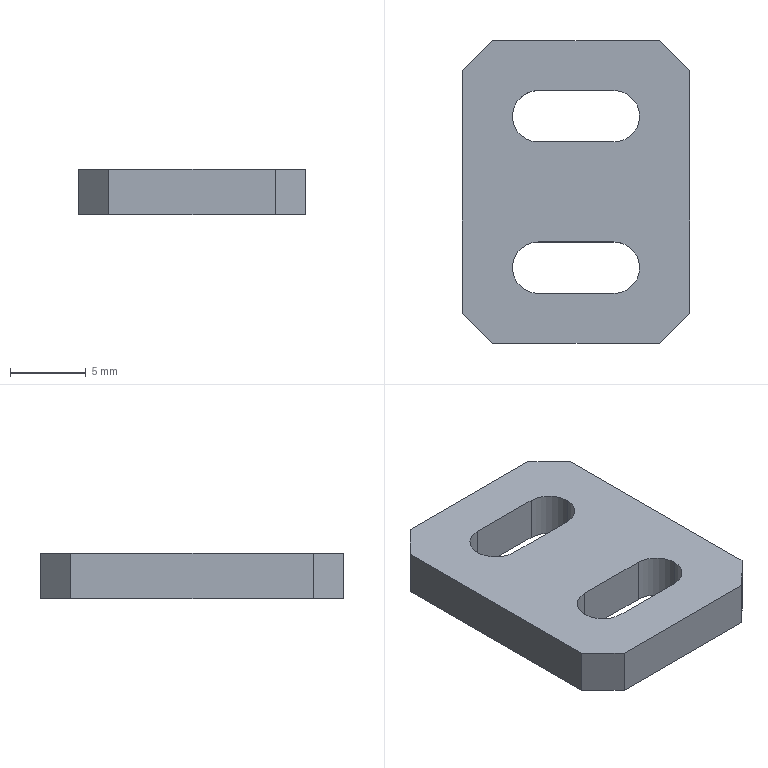Part | SolidWorks | features Chamfer 1, Extrusion 1, HoleWzd 1 | 1 solid | 20 faces | box 15 x 20 x 3 mm | volume 719.525 mm3 | plane 14 | cylinder 6 | commonest cylinder face diameters 3.4 x6
STEP:
#1=CARTESIAN_POINT('',(4.2,5.,0.));
#2=VERTEX_POINT('',#1);
#3=CARTESIAN_POINT('',(2.5,6.7,0.));
#4=VERTEX_POINT('',#3);
#5=CARTESIAN_POINT('',(2.5,5.,0.));
#6=DIRECTION('',(0.,0.,1.));
#7=DIRECTION('',(1.,0.,0.));
#8=AXIS2_PLACEMENT_3D('',#5,#6,#7);
#9=CIRCLE('',#8,1.7);
#10=EDGE_CURVE('',#2,#4,#9,.T.);
#11=ORIENTED_EDGE('',*,*,#10,.F.);
#12=CARTESIAN_POINT('',(4.2,5.,3.));
#13=VERTEX_POINT('',#12);
#14=CARTESIAN_POINT('',(4.2,5.,3.));
#15=DIRECTION('',(0.,0.,1.));
#16=VECTOR('',#15,1000.);
#17=LINE('',#14,#16);
#18=EDGE_CURVE('',#2,#13,#17,.T.);
#19=ORIENTED_EDGE('',*,*,#18,.T.);
#20=CARTESIAN_POINT('',(2.5,6.7,3.));
#21=VERTEX_POINT('',#20);
#22=CARTESIAN_POINT('',(2.5,5.,3.));
#23=DIRECTION('',(0.,0.,1.));
#24=DIRECTION('',(1.,0.,0.));
#25=AXIS2_PLACEMENT_3D('',#22,#23,#24);
#26=CIRCLE('',#25,1.7);
#27=EDGE_CURVE('',#13,#21,#26,.T.);
#28=ORIENTED_EDGE('',*,*,#27,.T.);
#29=CARTESIAN_POINT('',(2.5,6.7,3.));
#30=DIRECTION('',(0.,0.,1.));
#31=VECTOR('',#30,1000.);
#32=LINE('',#29,#31);
#33=EDGE_CURVE('',#4,#21,#32,.T.);
#34=ORIENTED_EDGE('',*,*,#33,.F.);
#35=EDGE_LOOP('',(#11,#19,#28,#34));
#36=FACE_OUTER_BOUND('',#35,.T.);
#37=CARTESIAN_POINT('',(2.5,5.,3.));
#38=DIRECTION('',(0.,0.,1.));
#39=DIRECTION('',(1.,0.,0.));
#40=AXIS2_PLACEMENT_3D('',#37,#38,#39);
#41=CYLINDRICAL_SURFACE('',#40,1.7);
#42=ADVANCED_FACE('',(#36),#41,.F.);
#43=CARTESIAN_POINT('',(4.2,-5.,0.));
#44=VERTEX_POINT('',#43);
#45=CARTESIAN_POINT('',(2.5,-3.3,0.));
#46=VERTEX_POINT('',#45);
#47=CARTESIAN_POINT('',(2.5,-5.,0.));
#48=DIRECTION('',(0.,0.,1.));
#49=DIRECTION('',(1.,0.,0.));
#50=AXIS2_PLACEMENT_3D('',#47,#48,#49);
#51=CIRCLE('',#50,1.7);
#52=EDGE_CURVE('',#44,#46,#51,.T.);
#53=ORIENTED_EDGE('',*,*,#52,.F.);
#54=CARTESIAN_POINT('',(4.2,-5.,3.));
#55=VERTEX_POINT('',#54);
#56=CARTESIAN_POINT('',(4.2,-5.,3.));
#57=DIRECTION('',(0.,0.,1.));
#58=VECTOR('',#57,1000.);
#59=LINE('',#56,#58);
#60=EDGE_CURVE('',#44,#55,#59,.T.);
#61=ORIENTED_EDGE('',*,*,#60,.T.);
#62=CARTESIAN_POINT('',(2.5,-3.3,3.));
#63=VERTEX_POINT('',#62);
#64=CARTESIAN_POINT('',(2.5,-5.,3.));
#65=DIRECTION('',(0.,0.,1.));
#66=DIRECTION('',(1.,0.,0.));
#67=AXIS2_PLACEMENT_3D('',#64,#65,#66);
#68=CIRCLE('',#67,1.7);
#69=EDGE_CURVE('',#55,#63,#68,.T.);
#70=ORIENTED_EDGE('',*,*,#69,.T.);
#71=CARTESIAN_POINT('',(2.5,-3.3,3.));
#72=DIRECTION('',(0.,0.,1.));
#73=VECTOR('',#72,1000.);
#74=LINE('',#71,#73);
#75=EDGE_CURVE('',#46,#63,#74,.T.);
#76=ORIENTED_EDGE('',*,*,#75,.F.);
#77=EDGE_LOOP('',(#53,#61,#70,#76));
#78=FACE_OUTER_BOUND('',#77,.T.);
#79=CARTESIAN_POINT('',(2.5,-5.,3.));
#80=DIRECTION('',(0.,0.,1.));
#81=DIRECTION('',(1.,0.,0.));
#82=AXIS2_PLACEMENT_3D('',#79,#80,#81);
#83=CYLINDRICAL_SURFACE('',#82,1.7);
#84=ADVANCED_FACE('',(#78),#83,.F.);
#85=CARTESIAN_POINT('',(7.5,-8.,0.));
#86=VERTEX_POINT('',#85);
#87=CARTESIAN_POINT('',(7.5,8.,0.));
#88=VERTEX_POINT('',#87);
#89=CARTESIAN_POINT('',(7.5,10.,0.));
#90=DIRECTION('',(0.,1.,0.));
#91=VECTOR('',#90,1000.);
#92=LINE('',#89,#91);
#93=EDGE_CURVE('',#86,#88,#92,.T.);
#94=ORIENTED_EDGE('',*,*,#93,.T.);
#95=CARTESIAN_POINT('',(7.5,8.,3.));
#96=VERTEX_POINT('',#95);
#97=CARTESIAN_POINT('',(7.5,8.,3.));
#98=DIRECTION('',(0.,0.,1.));
#99=VECTOR('',#98,1000.);
#100=LINE('',#97,#99);
#101=EDGE_CURVE('',#88,#96,#100,.T.);
#102=ORIENTED_EDGE('',*,*,#101,.T.);
#103=CARTESIAN_POINT('',(7.5,-8.,3.));
#104=VERTEX_POINT('',#103);
#105=CARTESIAN_POINT('',(7.5,10.,3.));
#106=DIRECTION('',(0.,1.,0.));
#107=VECTOR('',#106,1000.);
#108=LINE('',#105,#107);
#109=EDGE_CURVE('',#104,#96,#108,.T.);
#110=ORIENTED_EDGE('',*,*,#109,.F.);
#111=CARTESIAN_POINT('',(7.5,-8.,3.));
#112=DIRECTION('',(0.,0.,-1.));
#113=VECTOR('',#112,1000.);
#114=LINE('',#111,#113);
#115=EDGE_CURVE('',#104,#86,#114,.T.);
#116=ORIENTED_EDGE('',*,*,#115,.T.);
#117=EDGE_LOOP('',(#94,#102,#110,#116));
#118=FACE_OUTER_BOUND('',#117,.T.);
#119=CARTESIAN_POINT('',(7.5,10.,3.));
#120=DIRECTION('',(-1.,0.,0.));
#121=DIRECTION('',(0.,-1.,0.));
#122=AXIS2_PLACEMENT_3D('',#119,#120,#121);
#123=PLANE('',#122);
#124=ADVANCED_FACE('',(#118),#123,.F.);
#125=CARTESIAN_POINT('',(5.5,10.,3.));
#126=VERTEX_POINT('',#125);
#127=CARTESIAN_POINT('',(-5.5,10.,3.));
#128=VERTEX_POINT('',#127);
#129=CARTESIAN_POINT('',(-7.5,10.,3.));
#130=DIRECTION('',(-1.,0.,0.));
#131=VECTOR('',#130,1000.);
#132=LINE('',#129,#131);
#133=EDGE_CURVE('',#126,#128,#132,.T.);
#134=ORIENTED_EDGE('',*,*,#133,.F.);
#135=CARTESIAN_POINT('',(5.5,10.,0.));
#136=VERTEX_POINT('',#135);
#137=CARTESIAN_POINT('',(5.5,10.,3.));
#138=DIRECTION('',(0.,0.,-1.));
#139=VECTOR('',#138,1000.);
#140=LINE('',#137,#139);
#141=EDGE_CURVE('',#126,#136,#140,.T.);
#142=ORIENTED_EDGE('',*,*,#141,.T.);
#143=CARTESIAN_POINT('',(-5.5,10.,0.));
#144=VERTEX_POINT('',#143);
#145=CARTESIAN_POINT('',(-7.5,10.,0.));
#146=DIRECTION('',(-1.,0.,0.));
#147=VECTOR('',#146,1000.);
#148=LINE('',#145,#147);
#149=EDGE_CURVE('',#136,#144,#148,.T.);
#150=ORIENTED_EDGE('',*,*,#149,.T.);
#151=CARTESIAN_POINT('',(-5.5,10.,3.));
#152=DIRECTION('',(0.,0.,1.));
#153=VECTOR('',#152,1000.);
#154=LINE('',#151,#153);
#155=EDGE_CURVE('',#144,#128,#154,.T.);
#156=ORIENTED_EDGE('',*,*,#155,.T.);
#157=EDGE_LOOP('',(#134,#142,#150,#156));
#158=FACE_OUTER_BOUND('',#157,.T.);
#159=CARTESIAN_POINT('',(-7.5,10.,3.));
#160=DIRECTION('',(0.,-1.,0.));
#161=DIRECTION('',(0.,0.,-1.));
#162=AXIS2_PLACEMENT_3D('',#159,#160,#161);
#163=PLANE('',#162);
#164=ADVANCED_FACE('',(#158),#163,.F.);
#165=CARTESIAN_POINT('',(-7.5,8.,3.));
#166=VERTEX_POINT('',#165);
#167=CARTESIAN_POINT('',(-7.5,-8.,3.));
#168=VERTEX_POINT('',#167);
#169=CARTESIAN_POINT('',(-7.5,10.,3.));
#170=DIRECTION('',(0.,-1.,0.));
#171=VECTOR('',#170,1000.);
#172=LINE('',#169,#171);
#173=EDGE_CURVE('',#166,#168,#172,.T.);
#174=ORIENTED_EDGE('',*,*,#173,.F.);
#175=CARTESIAN_POINT('',(-7.5,8.,0.));
#176=VERTEX_POINT('',#175);
#177=CARTESIAN_POINT('',(-7.5,8.,3.));
#178=DIRECTION('',(0.,0.,-1.));
#179=VECTOR('',#178,1000.);
#180=LINE('',#177,#179);
#181=EDGE_CURVE('',#166,#176,#180,.T.);
#182=ORIENTED_EDGE('',*,*,#181,.T.);
#183=CARTESIAN_POINT('',(-7.5,-8.,0.));
#184=VERTEX_POINT('',#183);
#185=CARTESIAN_POINT('',(-7.5,10.,0.));
#186=DIRECTION('',(0.,-1.,0.));
#187=VECTOR('',#186,1000.);
#188=LINE('',#185,#187);
#189=EDGE_CURVE('',#176,#184,#188,.T.);
#190=ORIENTED_EDGE('',*,*,#189,.T.);
#191=CARTESIAN_POINT('',(-7.5,-8.,3.));
#192=DIRECTION('',(0.,0.,1.));
#193=VECTOR('',#192,1000.);
#194=LINE('',#191,#193);
#195=EDGE_CURVE('',#184,#168,#194,.T.);
#196=ORIENTED_EDGE('',*,*,#195,.T.);
#197=EDGE_LOOP('',(#174,#182,#190,#196));
#198=FACE_OUTER_BOUND('',#197,.T.);
#199=CARTESIAN_POINT('',(-7.5,10.,3.));
#200=DIRECTION('',(1.,0.,0.));
#201=DIRECTION('',(0.,1.,0.));
#202=AXIS2_PLACEMENT_3D('',#199,#200,#201);
#203=PLANE('',#202);
#204=ADVANCED_FACE('',(#198),#203,.F.);
#205=CARTESIAN_POINT('',(-5.5,-10.,3.));
#206=VERTEX_POINT('',#205);
#207=CARTESIAN_POINT('',(5.5,-10.,3.));
#208=VERTEX_POINT('',#207);
#209=CARTESIAN_POINT('',(-7.5,-10.,3.));
#210=DIRECTION('',(1.,0.,0.));
#211=VECTOR('',#210,1000.);
#212=LINE('',#209,#211);
#213=EDGE_CURVE('',#206,#208,#212,.T.);
#214=ORIENTED_EDGE('',*,*,#213,.F.);
#215=CARTESIAN_POINT('',(-5.5,-10.,0.));
#216=VERTEX_POINT('',#215);
#217=CARTESIAN_POINT('',(-5.5,-10.,3.));
#218=DIRECTION('',(0.,0.,-1.));
#219=VECTOR('',#218,1000.);
#220=LINE('',#217,#219);
#221=EDGE_CURVE('',#206,#216,#220,.T.);
#222=ORIENTED_EDGE('',*,*,#221,.T.);
#223=CARTESIAN_POINT('',(5.5,-10.,0.));
#224=VERTEX_POINT('',#223);
#225=CARTESIAN_POINT('',(-7.5,-10.,0.));
#226=DIRECTION('',(1.,0.,0.));
#227=VECTOR('',#226,1000.);
#228=LINE('',#225,#227);
#229=EDGE_CURVE('',#216,#224,#228,.T.);
#230=ORIENTED_EDGE('',*,*,#229,.T.);
#231=CARTESIAN_POINT('',(5.5,-10.,3.));
#232=DIRECTION('',(0.,0.,1.));
#233=VECTOR('',#232,1000.);
#234=LINE('',#231,#233);
#235=EDGE_CURVE('',#224,#208,#234,.T.);
#236=ORIENTED_EDGE('',*,*,#235,.T.);
#237=EDGE_LOOP('',(#214,#222,#230,#236));
#238=FACE_OUTER_BOUND('',#237,.T.);
#239=CARTESIAN_POINT('',(-7.5,-10.,3.));
#240=DIRECTION('',(0.,1.,0.));
#241=DIRECTION('',(0.,0.,1.));
#242=AXIS2_PLACEMENT_3D('',#239,#240,#241);
#243=PLANE('',#242);
#244=ADVANCED_FACE('',(#238),#243,.F.);
#245=CARTESIAN_POINT('',(-2.5,3.3,3.));
#246=VERTEX_POINT('',#245);
#247=CARTESIAN_POINT('',(2.5,3.3,3.));
#248=VERTEX_POINT('',#247);
#249=CARTESIAN_POINT('',(-2.5,3.3,3.));
#250=DIRECTION('',(1.,0.,0.));
#251=VECTOR('',#250,1000.);
#252=LINE('',#249,#251);
#253=EDGE_CURVE('',#246,#248,#252,.T.);
#254=ORIENTED_EDGE('',*,*,#253,.F.);
#255=CARTESIAN_POINT('',(-2.5,6.7,3.));
#256=VERTEX_POINT('',#255);
#257=CARTESIAN_POINT('',(-2.5,5.,3.));
#258=DIRECTION('',(0.,0.,1.));
#259=DIRECTION('',(1.,0.,0.));
#260=AXIS2_PLACEMENT_3D('',#257,#258,#259);
#261=CIRCLE('',#260,1.7);
#262=EDGE_CURVE('',#256,#246,#261,.T.);
#263=ORIENTED_EDGE('',*,*,#262,.F.);
#264=CARTESIAN_POINT('',(-2.5,6.7,3.));
#265=DIRECTION('',(1.,0.,0.));
#266=VECTOR('',#265,1000.);
#267=LINE('',#264,#266);
#268=EDGE_CURVE('',#256,#21,#267,.T.);
#269=ORIENTED_EDGE('',*,*,#268,.T.);
#270=ORIENTED_EDGE('',*,*,#27,.F.);
#271=CARTESIAN_POINT('',(2.5,5.,3.));
#272=DIRECTION('',(0.,0.,1.));
#273=DIRECTION('',(1.,0.,0.));
#274=AXIS2_PLACEMENT_3D('',#271,#272,#273);
#275=CIRCLE('',#274,1.7);
#276=EDGE_CURVE('',#248,#13,#275,.T.);
#277=ORIENTED_EDGE('',*,*,#276,.F.);
#278=EDGE_LOOP('',(#254,#263,#269,#270,#277));
#279=FACE_BOUND('',#278,.T.);
#280=CARTESIAN_POINT('',(-2.5,-3.3,3.));
#281=VERTEX_POINT('',#280);
#282=CARTESIAN_POINT('',(-2.5,-6.7,3.));
#283=VERTEX_POINT('',#282);
#284=CARTESIAN_POINT('',(-2.5,-5.,3.));
#285=DIRECTION('',(0.,0.,1.));
#286=DIRECTION('',(1.,0.,0.));
#287=AXIS2_PLACEMENT_3D('',#284,#285,#286);
#288=CIRCLE('',#287,1.7);
#289=EDGE_CURVE('',#281,#283,#288,.T.);
#290=ORIENTED_EDGE('',*,*,#289,.F.);
#291=CARTESIAN_POINT('',(-2.5,-3.3,3.));
#292=DIRECTION('',(1.,0.,0.));
#293=VECTOR('',#292,1000.);
#294=LINE('',#291,#293);
#295=EDGE_CURVE('',#281,#63,#294,.T.);
#296=ORIENTED_EDGE('',*,*,#295,.T.);
#297=ORIENTED_EDGE('',*,*,#69,.F.);
#298=CARTESIAN_POINT('',(2.5,-6.7,3.));
#299=VERTEX_POINT('',#298);
#300=CARTESIAN_POINT('',(2.5,-5.,3.));
#301=DIRECTION('',(0.,0.,1.));
#302=DIRECTION('',(1.,0.,0.));
#303=AXIS2_PLACEMENT_3D('',#300,#301,#302);
#304=CIRCLE('',#303,1.7);
#305=EDGE_CURVE('',#299,#55,#304,.T.);
#306=ORIENTED_EDGE('',*,*,#305,.F.);
#307=CARTESIAN_POINT('',(-2.5,-6.7,3.));
#308=DIRECTION('',(1.,0.,0.));
#309=VECTOR('',#308,1000.);
#310=LINE('',#307,#309);
#311=EDGE_CURVE('',#283,#299,#310,.T.);
#312=ORIENTED_EDGE('',*,*,#311,.F.);
#313=EDGE_LOOP('',(#290,#296,#297,#306,#312));
#314=FACE_BOUND('',#313,.T.);
#315=ORIENTED_EDGE('',*,*,#109,.T.);
#316=CARTESIAN_POINT('',(7.75,7.75,3.));
#317=DIRECTION('',(-0.7071,0.7071,0.));
#318=VECTOR('',#317,1000.);
#319=LINE('',#316,#318);
#320=EDGE_CURVE('',#96,#126,#319,.T.);
#321=ORIENTED_EDGE('',*,*,#320,.T.);
#322=ORIENTED_EDGE('',*,*,#133,.T.);
#323=CARTESIAN_POINT('',(-7.75,7.75,3.));
#324=DIRECTION('',(-0.7071,-0.7071,0.));
#325=VECTOR('',#324,1000.);
#326=LINE('',#323,#325);
#327=EDGE_CURVE('',#128,#166,#326,.T.);
#328=ORIENTED_EDGE('',*,*,#327,.T.);
#329=ORIENTED_EDGE('',*,*,#173,.T.);
#330=CARTESIAN_POINT('',(-7.75,-7.75,3.));
#331=DIRECTION('',(0.7071,-0.7071,0.));
#332=VECTOR('',#331,1000.);
#333=LINE('',#330,#332);
#334=EDGE_CURVE('',#168,#206,#333,.T.);
#335=ORIENTED_EDGE('',*,*,#334,.T.);
#336=ORIENTED_EDGE('',*,*,#213,.T.);
#337=CARTESIAN_POINT('',(7.75,-7.75,3.));
#338=DIRECTION('',(0.7071,0.7071,0.));
#339=VECTOR('',#338,1000.);
#340=LINE('',#337,#339);
#341=EDGE_CURVE('',#208,#104,#340,.T.);
#342=ORIENTED_EDGE('',*,*,#341,.T.);
#343=EDGE_LOOP('',(#315,#321,#322,#328,#329,#335,#336,#342));
#344=FACE_OUTER_BOUND('',#343,.T.);
#345=CARTESIAN_POINT('',(0.,0.,3.));
#346=DIRECTION('',(0.,0.,1.));
#347=DIRECTION('',(1.,0.,0.));
#348=AXIS2_PLACEMENT_3D('',#345,#346,#347);
#349=PLANE('',#348);
#350=ADVANCED_FACE('',(#279,#314,#344),#349,.T.);
#351=CARTESIAN_POINT('',(-2.5,6.7,0.));
#352=VERTEX_POINT('',#351);
#353=CARTESIAN_POINT('',(-2.5,6.7,0.));
#354=DIRECTION('',(1.,0.,0.));
#355=VECTOR('',#354,1000.);
#356=LINE('',#353,#355);
#357=EDGE_CURVE('',#352,#4,#356,.T.);
#358=ORIENTED_EDGE('',*,*,#357,.F.);
#359=CARTESIAN_POINT('',(-2.5,3.3,0.));
#360=VERTEX_POINT('',#359);
#361=CARTESIAN_POINT('',(-2.5,5.,0.));
#362=DIRECTION('',(0.,0.,1.));
#363=DIRECTION('',(1.,0.,0.));
#364=AXIS2_PLACEMENT_3D('',#361,#362,#363);
#365=CIRCLE('',#364,1.7);
#366=EDGE_CURVE('',#352,#360,#365,.T.);
#367=ORIENTED_EDGE('',*,*,#366,.T.);
#368=CARTESIAN_POINT('',(2.5,3.3,0.));
#369=VERTEX_POINT('',#368);
#370=CARTESIAN_POINT('',(-2.5,3.3,0.));
#371=DIRECTION('',(1.,0.,0.));
#372=VECTOR('',#371,1000.);
#373=LINE('',#370,#372);
#374=EDGE_CURVE('',#360,#369,#373,.T.);
#375=ORIENTED_EDGE('',*,*,#374,.T.);
#376=CARTESIAN_POINT('',(2.5,5.,0.));
#377=DIRECTION('',(0.,0.,1.));
#378=DIRECTION('',(1.,0.,0.));
#379=AXIS2_PLACEMENT_3D('',#376,#377,#378);
#380=CIRCLE('',#379,1.7);
#381=EDGE_CURVE('',#369,#2,#380,.T.);
#382=ORIENTED_EDGE('',*,*,#381,.T.);
#383=ORIENTED_EDGE('',*,*,#10,.T.);
#384=EDGE_LOOP('',(#358,#367,#375,#382,#383));
#385=FACE_BOUND('',#384,.T.);
#386=CARTESIAN_POINT('',(-2.5,-3.3,0.));
#387=VERTEX_POINT('',#386);
#388=CARTESIAN_POINT('',(-2.5,-6.7,0.));
#389=VERTEX_POINT('',#388);
#390=CARTESIAN_POINT('',(-2.5,-5.,0.));
#391=DIRECTION('',(0.,0.,1.));
#392=DIRECTION('',(1.,0.,0.));
#393=AXIS2_PLACEMENT_3D('',#390,#391,#392);
#394=CIRCLE('',#393,1.7);
#395=EDGE_CURVE('',#387,#389,#394,.T.);
#396=ORIENTED_EDGE('',*,*,#395,.T.);
#397=CARTESIAN_POINT('',(2.5,-6.7,0.));
#398=VERTEX_POINT('',#397);
#399=CARTESIAN_POINT('',(-2.5,-6.7,0.));
#400=DIRECTION('',(1.,0.,0.));
#401=VECTOR('',#400,1000.);
#402=LINE('',#399,#401);
#403=EDGE_CURVE('',#389,#398,#402,.T.);
#404=ORIENTED_EDGE('',*,*,#403,.T.);
#405=CARTESIAN_POINT('',(2.5,-5.,0.));
#406=DIRECTION('',(0.,0.,1.));
#407=DIRECTION('',(1.,0.,0.));
#408=AXIS2_PLACEMENT_3D('',#405,#406,#407);
#409=CIRCLE('',#408,1.7);
#410=EDGE_CURVE('',#398,#44,#409,.T.);
#411=ORIENTED_EDGE('',*,*,#410,.T.);
#412=ORIENTED_EDGE('',*,*,#52,.T.);
#413=CARTESIAN_POINT('',(-2.5,-3.3,0.));
#414=DIRECTION('',(1.,0.,0.));
#415=VECTOR('',#414,1000.);
#416=LINE('',#413,#415);
#417=EDGE_CURVE('',#387,#46,#416,.T.);
#418=ORIENTED_EDGE('',*,*,#417,.F.);
#419=EDGE_LOOP('',(#396,#404,#411,#412,#418));
#420=FACE_BOUND('',#419,.T.);
#421=ORIENTED_EDGE('',*,*,#149,.F.);
#422=CARTESIAN_POINT('',(5.5,10.,0.));
#423=DIRECTION('',(0.7071,-0.7071,0.));
#424=VECTOR('',#423,1000.);
#425=LINE('',#422,#424);
#426=EDGE_CURVE('',#136,#88,#425,.T.);
#427=ORIENTED_EDGE('',*,*,#426,.T.);
#428=ORIENTED_EDGE('',*,*,#93,.F.);
#429=CARTESIAN_POINT('',(7.5,-8.,0.));
#430=DIRECTION('',(-0.7071,-0.7071,0.));
#431=VECTOR('',#430,1000.);
#432=LINE('',#429,#431);
#433=EDGE_CURVE('',#86,#224,#432,.T.);
#434=ORIENTED_EDGE('',*,*,#433,.T.);
#435=ORIENTED_EDGE('',*,*,#229,.F.);
#436=CARTESIAN_POINT('',(-5.5,-10.,0.));
#437=DIRECTION('',(-0.7071,0.7071,0.));
#438=VECTOR('',#437,1000.);
#439=LINE('',#436,#438);
#440=EDGE_CURVE('',#216,#184,#439,.T.);
#441=ORIENTED_EDGE('',*,*,#440,.T.);
#442=ORIENTED_EDGE('',*,*,#189,.F.);
#443=CARTESIAN_POINT('',(-7.5,8.,0.));
#444=DIRECTION('',(0.7071,0.7071,0.));
#445=VECTOR('',#444,1000.);
#446=LINE('',#443,#445);
#447=EDGE_CURVE('',#176,#144,#446,.T.);
#448=ORIENTED_EDGE('',*,*,#447,.T.);
#449=EDGE_LOOP('',(#421,#427,#428,#434,#435,#441,#442,#448));
#450=FACE_OUTER_BOUND('',#449,.T.);
#451=CARTESIAN_POINT('',(0.,0.,0.));
#452=DIRECTION('',(0.,0.,1.));
#453=DIRECTION('',(1.,0.,0.));
#454=AXIS2_PLACEMENT_3D('',#451,#452,#453);
#455=PLANE('',#454);
#456=ADVANCED_FACE('',(#385,#420,#450),#455,.F.);
#457=ORIENTED_EDGE('',*,*,#60,.F.);
#458=ORIENTED_EDGE('',*,*,#410,.F.);
#459=CARTESIAN_POINT('',(2.5,-6.7,3.));
#460=DIRECTION('',(0.,0.,-1.));
#461=VECTOR('',#460,1000.);
#462=LINE('',#459,#461);
#463=EDGE_CURVE('',#299,#398,#462,.T.);
#464=ORIENTED_EDGE('',*,*,#463,.F.);
#465=ORIENTED_EDGE('',*,*,#305,.T.);
#466=EDGE_LOOP('',(#457,#458,#464,#465));
#467=FACE_OUTER_BOUND('',#466,.T.);
#468=CARTESIAN_POINT('',(2.5,-5.,3.));
#469=DIRECTION('',(0.,0.,1.));
#470=DIRECTION('',(1.,0.,0.));
#471=AXIS2_PLACEMENT_3D('',#468,#469,#470);
#472=CYLINDRICAL_SURFACE('',#471,1.7);
#473=ADVANCED_FACE('',(#467),#472,.F.);
#474=ORIENTED_EDGE('',*,*,#289,.T.);
#475=CARTESIAN_POINT('',(-2.5,-6.7,3.));
#476=DIRECTION('',(0.,0.,1.));
#477=VECTOR('',#476,1000.);
#478=LINE('',#475,#477);
#479=EDGE_CURVE('',#389,#283,#478,.T.);
#480=ORIENTED_EDGE('',*,*,#479,.F.);
#481=ORIENTED_EDGE('',*,*,#395,.F.);
#482=CARTESIAN_POINT('',(-2.5,-3.3,3.));
#483=DIRECTION('',(0.,0.,-1.));
#484=VECTOR('',#483,1000.);
#485=LINE('',#482,#484);
#486=EDGE_CURVE('',#281,#387,#485,.T.);
#487=ORIENTED_EDGE('',*,*,#486,.F.);
#488=EDGE_LOOP('',(#474,#480,#481,#487));
#489=FACE_OUTER_BOUND('',#488,.T.);
#490=CARTESIAN_POINT('',(-2.5,-5.,3.));
#491=DIRECTION('',(0.,0.,1.));
#492=DIRECTION('',(1.,0.,0.));
#493=AXIS2_PLACEMENT_3D('',#490,#491,#492);
#494=CYLINDRICAL_SURFACE('',#493,1.7);
#495=ADVANCED_FACE('',(#489),#494,.F.);
#496=ORIENTED_EDGE('',*,*,#75,.T.);
#497=ORIENTED_EDGE('',*,*,#295,.F.);
#498=ORIENTED_EDGE('',*,*,#486,.T.);
#499=ORIENTED_EDGE('',*,*,#417,.T.);
#500=EDGE_LOOP('',(#496,#497,#498,#499));
#501=FACE_OUTER_BOUND('',#500,.T.);
#502=CARTESIAN_POINT('',(-2.5,-3.3,3.));
#503=DIRECTION('',(0.,1.,0.));
#504=DIRECTION('',(-1.,0.,0.));
#505=AXIS2_PLACEMENT_3D('',#502,#503,#504);
#506=PLANE('',#505);
#507=ADVANCED_FACE('',(#501),#506,.F.);
#508=ORIENTED_EDGE('',*,*,#463,.T.);
#509=ORIENTED_EDGE('',*,*,#403,.F.);
#510=ORIENTED_EDGE('',*,*,#479,.T.);
#511=ORIENTED_EDGE('',*,*,#311,.T.);
#512=EDGE_LOOP('',(#508,#509,#510,#511));
#513=FACE_OUTER_BOUND('',#512,.T.);
#514=CARTESIAN_POINT('',(-2.5,-6.7,3.));
#515=DIRECTION('',(0.,-1.,0.));
#516=DIRECTION('',(1.,0.,0.));
#517=AXIS2_PLACEMENT_3D('',#514,#515,#516);
#518=PLANE('',#517);
#519=ADVANCED_FACE('',(#513),#518,.F.);
#520=ORIENTED_EDGE('',*,*,#18,.F.);
#521=ORIENTED_EDGE('',*,*,#381,.F.);
#522=CARTESIAN_POINT('',(2.5,3.3,3.));
#523=DIRECTION('',(0.,0.,-1.));
#524=VECTOR('',#523,1000.);
#525=LINE('',#522,#524);
#526=EDGE_CURVE('',#248,#369,#525,.T.);
#527=ORIENTED_EDGE('',*,*,#526,.F.);
#528=ORIENTED_EDGE('',*,*,#276,.T.);
#529=EDGE_LOOP('',(#520,#521,#527,#528));
#530=FACE_OUTER_BOUND('',#529,.T.);
#531=CARTESIAN_POINT('',(2.5,5.,3.));
#532=DIRECTION('',(0.,0.,1.));
#533=DIRECTION('',(1.,0.,0.));
#534=AXIS2_PLACEMENT_3D('',#531,#532,#533);
#535=CYLINDRICAL_SURFACE('',#534,1.7);
#536=ADVANCED_FACE('',(#530),#535,.F.);
#537=ORIENTED_EDGE('',*,*,#262,.T.);
#538=CARTESIAN_POINT('',(-2.5,3.3,3.));
#539=DIRECTION('',(0.,0.,1.));
#540=VECTOR('',#539,1000.);
#541=LINE('',#538,#540);
#542=EDGE_CURVE('',#360,#246,#541,.T.);
#543=ORIENTED_EDGE('',*,*,#542,.F.);
#544=ORIENTED_EDGE('',*,*,#366,.F.);
#545=CARTESIAN_POINT('',(-2.5,6.7,3.));
#546=DIRECTION('',(0.,0.,-1.));
#547=VECTOR('',#546,1000.);
#548=LINE('',#545,#547);
#549=EDGE_CURVE('',#256,#352,#548,.T.);
#550=ORIENTED_EDGE('',*,*,#549,.F.);
#551=EDGE_LOOP('',(#537,#543,#544,#550));
#552=FACE_OUTER_BOUND('',#551,.T.);
#553=CARTESIAN_POINT('',(-2.5,5.,3.));
#554=DIRECTION('',(0.,0.,1.));
#555=DIRECTION('',(1.,0.,0.));
#556=AXIS2_PLACEMENT_3D('',#553,#554,#555);
#557=CYLINDRICAL_SURFACE('',#556,1.7);
#558=ADVANCED_FACE('',(#552),#557,.F.);
#559=ORIENTED_EDGE('',*,*,#33,.T.);
#560=ORIENTED_EDGE('',*,*,#268,.F.);
#561=ORIENTED_EDGE('',*,*,#549,.T.);
#562=ORIENTED_EDGE('',*,*,#357,.T.);
#563=EDGE_LOOP('',(#559,#560,#561,#562));
#564=FACE_OUTER_BOUND('',#563,.T.);
#565=CARTESIAN_POINT('',(-2.5,6.7,3.));
#566=DIRECTION('',(0.,1.,0.));
#567=DIRECTION('',(-1.,0.,0.));
#568=AXIS2_PLACEMENT_3D('',#565,#566,#567);
#569=PLANE('',#568);
#570=ADVANCED_FACE('',(#564),#569,.F.);
#571=ORIENTED_EDGE('',*,*,#526,.T.);
#572=ORIENTED_EDGE('',*,*,#374,.F.);
#573=ORIENTED_EDGE('',*,*,#542,.T.);
#574=ORIENTED_EDGE('',*,*,#253,.T.);
#575=EDGE_LOOP('',(#571,#572,#573,#574));
#576=FACE_OUTER_BOUND('',#575,.T.);
#577=CARTESIAN_POINT('',(-2.5,3.3,3.));
#578=DIRECTION('',(0.,-1.,0.));
#579=DIRECTION('',(1.,0.,0.));
#580=AXIS2_PLACEMENT_3D('',#577,#578,#579);
#581=PLANE('',#580);
#582=ADVANCED_FACE('',(#576),#581,.F.);
#583=ORIENTED_EDGE('',*,*,#320,.F.);
#584=ORIENTED_EDGE('',*,*,#101,.F.);
#585=ORIENTED_EDGE('',*,*,#426,.F.);
#586=ORIENTED_EDGE('',*,*,#141,.F.);
#587=EDGE_LOOP('',(#583,#584,#585,#586));
#588=FACE_OUTER_BOUND('',#587,.T.);
#589=CARTESIAN_POINT('',(5.5,10.,3.));
#590=DIRECTION('',(-0.7071,-0.7071,0.));
#591=DIRECTION('',(0.,0.,-1.));
#592=AXIS2_PLACEMENT_3D('',#589,#590,#591);
#593=PLANE('',#592);
#594=ADVANCED_FACE('',(#588),#593,.F.);
#595=ORIENTED_EDGE('',*,*,#327,.F.);
#596=ORIENTED_EDGE('',*,*,#155,.F.);
#597=ORIENTED_EDGE('',*,*,#447,.F.);
#598=ORIENTED_EDGE('',*,*,#181,.F.);
#599=EDGE_LOOP('',(#595,#596,#597,#598));
#600=FACE_OUTER_BOUND('',#599,.T.);
#601=CARTESIAN_POINT('',(-7.5,8.,3.));
#602=DIRECTION('',(0.7071,-0.7071,0.));
#603=DIRECTION('',(0.,0.,-1.));
#604=AXIS2_PLACEMENT_3D('',#601,#602,#603);
#605=PLANE('',#604);
#606=ADVANCED_FACE('',(#600),#605,.F.);
#607=ORIENTED_EDGE('',*,*,#334,.F.);
#608=ORIENTED_EDGE('',*,*,#195,.F.);
#609=ORIENTED_EDGE('',*,*,#440,.F.);
#610=ORIENTED_EDGE('',*,*,#221,.F.);
#611=EDGE_LOOP('',(#607,#608,#609,#610));
#612=FACE_OUTER_BOUND('',#611,.T.);
#613=CARTESIAN_POINT('',(-5.5,-10.,3.));
#614=DIRECTION('',(0.7071,0.7071,0.));
#615=DIRECTION('',(0.,0.,-1.));
#616=AXIS2_PLACEMENT_3D('',#613,#614,#615);
#617=PLANE('',#616);
#618=ADVANCED_FACE('',(#612),#617,.F.);
#619=ORIENTED_EDGE('',*,*,#341,.F.);
#620=ORIENTED_EDGE('',*,*,#235,.F.);
#621=ORIENTED_EDGE('',*,*,#433,.F.);
#622=ORIENTED_EDGE('',*,*,#115,.F.);
#623=EDGE_LOOP('',(#619,#620,#621,#622));
#624=FACE_OUTER_BOUND('',#623,.T.);
#625=CARTESIAN_POINT('',(7.5,-8.,3.));
#626=DIRECTION('',(-0.7071,0.7071,0.));
#627=DIRECTION('',(0.,0.,-1.));
#628=AXIS2_PLACEMENT_3D('',#625,#626,#627);
#629=PLANE('',#628);
#630=ADVANCED_FACE('',(#624),#629,.F.);
#631=CLOSED_SHELL('',(#42,#84,#124,#164,#204,#244,#350,#456,#473,#495,#507,#519,#536,#558,#570,#582,#594,#606,#618,#630));
#632=MANIFOLD_SOLID_BREP('',#631);
#633=CARTESIAN_POINT('',(0.,0.,0.));
#634=DIRECTION('',(0.,0.,1.));
#635=DIRECTION('',(1.,0.,0.));
#636=AXIS2_PLACEMENT_3D('',#633,#634,#635);
#637=(LENGTH_UNIT()NAMED_UNIT(*)SI_UNIT(.MILLI.,.METRE.));
#638=UNCERTAINTY_MEASURE_WITH_UNIT(LENGTH_MEASURE(0.00001),#637,'','');
#639=(NAMED_UNIT(*)PLANE_ANGLE_UNIT()SI_UNIT($,.RADIAN.));
#640=(NAMED_UNIT(*)SI_UNIT($,.STERADIAN.)SOLID_ANGLE_UNIT());
#641=(GEOMETRIC_REPRESENTATION_CONTEXT(3)GLOBAL_UNCERTAINTY_ASSIGNED_CONTEXT((#638))GLOBAL_UNIT_ASSIGNED_CONTEXT((#637,#639,#640))REPRESENTATION_CONTEXT('',''));
#642=ADVANCED_BREP_SHAPE_REPRESENTATION('',(#632,#636),#641);